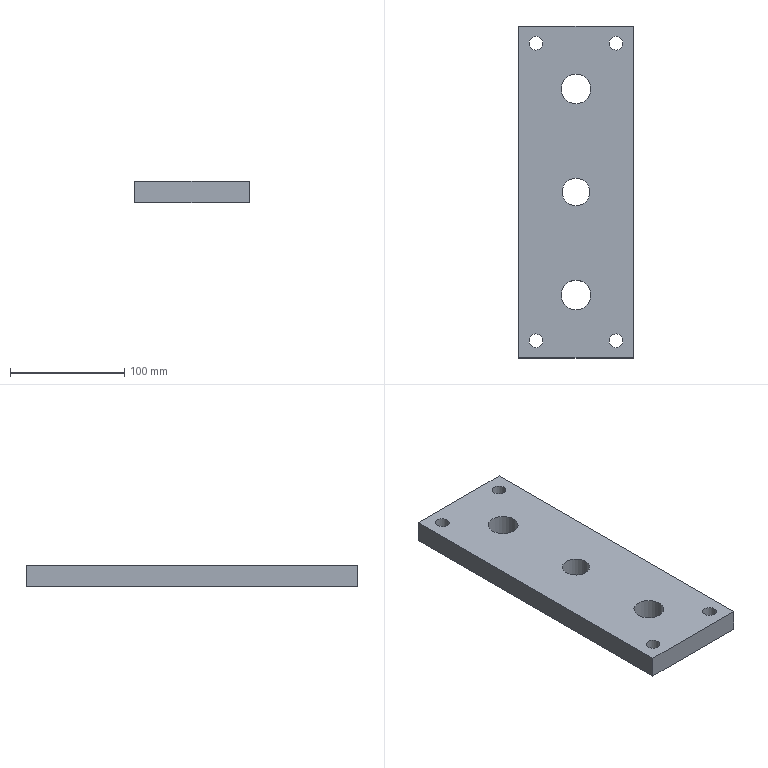Part | NX | features solid 2 | 1 solid | 13 faces | box 100 x 290 x 19 mm | volume 513634 mm3 | cylinder 7 | plane 6 | commonest cylinder face diameters 12 x4 26 x2 24 x1
STEP:
#1=CARTESIAN_POINT('',(235.,-226.,-122.));
#2=VERTEX_POINT('',#1);
#3=CARTESIAN_POINT('',(235.,-220.,-122.));
#4=DIRECTION('',(0.,0.,1.));
#5=DIRECTION('',(0.,-1.,0.));
#6=AXIS2_PLACEMENT_3D('',#3,#4,#5);
#7=CIRCLE('',#6,6.);
#8=EDGE_CURVE('',#2,#2,#7,.T.);
#9=ORIENTED_EDGE('',*,*,#8,.F.);
#10=EDGE_LOOP('',(#9));
#11=FACE_BOUND('',#10,.T.);
#12=CARTESIAN_POINT('',(235.,46.,-122.));
#13=VERTEX_POINT('',#12);
#14=CARTESIAN_POINT('',(235.,40.,-122.));
#15=DIRECTION('',(0.,0.,-1.));
#16=DIRECTION('',(0.,1.,0.));
#17=AXIS2_PLACEMENT_3D('',#14,#15,#16);
#18=CIRCLE('',#17,6.);
#19=EDGE_CURVE('',#13,#13,#18,.T.);
#20=ORIENTED_EDGE('',*,*,#19,.T.);
#21=EDGE_LOOP('',(#20));
#22=FACE_BOUND('',#21,.T.);
#23=CARTESIAN_POINT('',(250.,-235.,-122.));
#24=VERTEX_POINT('',#23);
#25=CARTESIAN_POINT('',(150.,-235.,-122.));
#26=VERTEX_POINT('',#25);
#27=CARTESIAN_POINT('',(250.,-235.,-122.));
#28=DIRECTION('',(-1.,0.,0.));
#29=VECTOR('',#28,1000.);
#30=LINE('',#27,#29);
#31=EDGE_CURVE('',#24,#26,#30,.T.);
#32=ORIENTED_EDGE('',*,*,#31,.F.);
#33=CARTESIAN_POINT('',(250.,55.,-122.));
#34=VERTEX_POINT('',#33);
#35=CARTESIAN_POINT('',(250.,55.,-122.));
#36=DIRECTION('',(0.,-1.,0.));
#37=VECTOR('',#36,1000.);
#38=LINE('',#35,#37);
#39=EDGE_CURVE('',#34,#24,#38,.T.);
#40=ORIENTED_EDGE('',*,*,#39,.F.);
#41=CARTESIAN_POINT('',(150.,55.,-122.));
#42=VERTEX_POINT('',#41);
#43=CARTESIAN_POINT('',(150.,55.,-122.));
#44=DIRECTION('',(1.,0.,0.));
#45=VECTOR('',#44,1000.);
#46=LINE('',#43,#45);
#47=EDGE_CURVE('',#42,#34,#46,.T.);
#48=ORIENTED_EDGE('',*,*,#47,.F.);
#49=CARTESIAN_POINT('',(150.,-235.,-122.));
#50=DIRECTION('',(0.,1.,0.));
#51=VECTOR('',#50,1000.);
#52=LINE('',#49,#51);
#53=EDGE_CURVE('',#26,#42,#52,.T.);
#54=ORIENTED_EDGE('',*,*,#53,.F.);
#55=EDGE_LOOP('',(#32,#40,#48,#54));
#56=FACE_BOUND('',#55,.T.);
#57=CARTESIAN_POINT('',(200.,-193.,-122.));
#58=VERTEX_POINT('',#57);
#59=CARTESIAN_POINT('',(200.,-180.,-122.));
#60=DIRECTION('',(0.,0.,1.));
#61=DIRECTION('',(0.,-1.,0.));
#62=AXIS2_PLACEMENT_3D('',#59,#60,#61);
#63=CIRCLE('',#62,13.);
#64=EDGE_CURVE('',#58,#58,#63,.F.);
#65=ORIENTED_EDGE('',*,*,#64,.T.);
#66=EDGE_LOOP('',(#65));
#67=FACE_BOUND('',#66,.T.);
#68=CARTESIAN_POINT('',(200.,-102.,-122.));
#69=VERTEX_POINT('',#68);
#70=CARTESIAN_POINT('',(200.,-90.,-122.));
#71=DIRECTION('',(0.,0.,1.));
#72=DIRECTION('',(0.,-1.,0.));
#73=AXIS2_PLACEMENT_3D('',#70,#71,#72);
#74=CIRCLE('',#73,12.);
#75=EDGE_CURVE('',#69,#69,#74,.F.);
#76=ORIENTED_EDGE('',*,*,#75,.T.);
#77=EDGE_LOOP('',(#76));
#78=FACE_BOUND('',#77,.T.);
#79=CARTESIAN_POINT('',(165.,46.,-122.));
#80=VERTEX_POINT('',#79);
#81=CARTESIAN_POINT('',(165.,40.,-122.));
#82=DIRECTION('',(0.,0.,1.));
#83=DIRECTION('',(0.,1.,0.));
#84=AXIS2_PLACEMENT_3D('',#81,#82,#83);
#85=CIRCLE('',#84,6.);
#86=EDGE_CURVE('',#80,#80,#85,.T.);
#87=ORIENTED_EDGE('',*,*,#86,.F.);
#88=EDGE_LOOP('',(#87));
#89=FACE_BOUND('',#88,.T.);
#90=CARTESIAN_POINT('',(165.,-226.,-122.));
#91=VERTEX_POINT('',#90);
#92=CARTESIAN_POINT('',(165.,-220.,-122.));
#93=DIRECTION('',(0.,0.,-1.));
#94=DIRECTION('',(0.,-1.,0.));
#95=AXIS2_PLACEMENT_3D('',#92,#93,#94);
#96=CIRCLE('',#95,6.);
#97=EDGE_CURVE('',#91,#91,#96,.T.);
#98=ORIENTED_EDGE('',*,*,#97,.T.);
#99=EDGE_LOOP('',(#98));
#100=FACE_BOUND('',#99,.T.);
#101=CARTESIAN_POINT('',(200.,13.,-122.));
#102=VERTEX_POINT('',#101);
#103=CARTESIAN_POINT('',(200.,0.,-122.));
#104=DIRECTION('',(0.,0.,1.));
#105=DIRECTION('',(0.,1.,0.));
#106=AXIS2_PLACEMENT_3D('',#103,#104,#105);
#107=CIRCLE('',#106,13.);
#108=EDGE_CURVE('',#102,#102,#107,.T.);
#109=ORIENTED_EDGE('',*,*,#108,.F.);
#110=EDGE_LOOP('',(#109));
#111=FACE_BOUND('',#110,.T.);
#112=CARTESIAN_POINT('',(250.,-235.,-122.));
#113=DIRECTION('',(0.,0.,1.));
#114=DIRECTION('',(0.,-1.,0.));
#115=AXIS2_PLACEMENT_3D('',#112,#113,#114);
#116=PLANE('',#115);
#117=ADVANCED_FACE('',(#11,#22,#56,#67,#78,#89,#100,#111),#116,.T.);
#118=CARTESIAN_POINT('',(235.,-226.,-141.));
#119=VERTEX_POINT('',#118);
#120=CARTESIAN_POINT('',(235.,-220.,-141.));
#121=DIRECTION('',(0.,0.,1.));
#122=DIRECTION('',(0.,-1.,0.));
#123=AXIS2_PLACEMENT_3D('',#120,#121,#122);
#124=CIRCLE('',#123,6.);
#125=EDGE_CURVE('',#119,#119,#124,.T.);
#126=ORIENTED_EDGE('',*,*,#125,.T.);
#127=EDGE_LOOP('',(#126));
#128=FACE_BOUND('',#127,.T.);
#129=CARTESIAN_POINT('',(235.,46.,-141.));
#130=VERTEX_POINT('',#129);
#131=CARTESIAN_POINT('',(235.,40.,-141.));
#132=DIRECTION('',(0.,0.,-1.));
#133=DIRECTION('',(0.,1.,0.));
#134=AXIS2_PLACEMENT_3D('',#131,#132,#133);
#135=CIRCLE('',#134,6.);
#136=EDGE_CURVE('',#130,#130,#135,.T.);
#137=ORIENTED_EDGE('',*,*,#136,.F.);
#138=EDGE_LOOP('',(#137));
#139=FACE_BOUND('',#138,.T.);
#140=CARTESIAN_POINT('',(250.,-235.,-141.));
#141=VERTEX_POINT('',#140);
#142=CARTESIAN_POINT('',(150.,-235.,-141.));
#143=VERTEX_POINT('',#142);
#144=CARTESIAN_POINT('',(250.,-235.,-141.));
#145=DIRECTION('',(-1.,0.,0.));
#146=VECTOR('',#145,1000.);
#147=LINE('',#144,#146);
#148=EDGE_CURVE('',#141,#143,#147,.T.);
#149=ORIENTED_EDGE('',*,*,#148,.T.);
#150=CARTESIAN_POINT('',(150.,55.,-141.));
#151=VERTEX_POINT('',#150);
#152=CARTESIAN_POINT('',(150.,-235.,-141.));
#153=DIRECTION('',(0.,1.,0.));
#154=VECTOR('',#153,1000.);
#155=LINE('',#152,#154);
#156=EDGE_CURVE('',#143,#151,#155,.T.);
#157=ORIENTED_EDGE('',*,*,#156,.T.);
#158=CARTESIAN_POINT('',(250.,55.,-141.));
#159=VERTEX_POINT('',#158);
#160=CARTESIAN_POINT('',(150.,55.,-141.));
#161=DIRECTION('',(1.,0.,0.));
#162=VECTOR('',#161,1000.);
#163=LINE('',#160,#162);
#164=EDGE_CURVE('',#151,#159,#163,.T.);
#165=ORIENTED_EDGE('',*,*,#164,.T.);
#166=CARTESIAN_POINT('',(250.,55.,-141.));
#167=DIRECTION('',(0.,-1.,0.));
#168=VECTOR('',#167,1000.);
#169=LINE('',#166,#168);
#170=EDGE_CURVE('',#159,#141,#169,.T.);
#171=ORIENTED_EDGE('',*,*,#170,.T.);
#172=EDGE_LOOP('',(#149,#157,#165,#171));
#173=FACE_BOUND('',#172,.T.);
#174=CARTESIAN_POINT('',(200.,-193.,-141.));
#175=VERTEX_POINT('',#174);
#176=CARTESIAN_POINT('',(200.,-180.,-141.));
#177=DIRECTION('',(0.,0.,1.));
#178=DIRECTION('',(0.,-1.,0.));
#179=AXIS2_PLACEMENT_3D('',#176,#177,#178);
#180=CIRCLE('',#179,13.);
#181=EDGE_CURVE('',#175,#175,#180,.F.);
#182=ORIENTED_EDGE('',*,*,#181,.F.);
#183=EDGE_LOOP('',(#182));
#184=FACE_BOUND('',#183,.T.);
#185=CARTESIAN_POINT('',(200.,-102.,-141.));
#186=VERTEX_POINT('',#185);
#187=CARTESIAN_POINT('',(200.,-90.,-141.));
#188=DIRECTION('',(0.,0.,1.));
#189=DIRECTION('',(0.,-1.,0.));
#190=AXIS2_PLACEMENT_3D('',#187,#188,#189);
#191=CIRCLE('',#190,12.);
#192=EDGE_CURVE('',#186,#186,#191,.F.);
#193=ORIENTED_EDGE('',*,*,#192,.F.);
#194=EDGE_LOOP('',(#193));
#195=FACE_BOUND('',#194,.T.);
#196=CARTESIAN_POINT('',(165.,46.,-141.));
#197=VERTEX_POINT('',#196);
#198=CARTESIAN_POINT('',(165.,40.,-141.));
#199=DIRECTION('',(0.,0.,1.));
#200=DIRECTION('',(0.,1.,0.));
#201=AXIS2_PLACEMENT_3D('',#198,#199,#200);
#202=CIRCLE('',#201,6.);
#203=EDGE_CURVE('',#197,#197,#202,.T.);
#204=ORIENTED_EDGE('',*,*,#203,.T.);
#205=EDGE_LOOP('',(#204));
#206=FACE_BOUND('',#205,.T.);
#207=CARTESIAN_POINT('',(165.,-226.,-141.));
#208=VERTEX_POINT('',#207);
#209=CARTESIAN_POINT('',(165.,-220.,-141.));
#210=DIRECTION('',(0.,0.,-1.));
#211=DIRECTION('',(0.,-1.,0.));
#212=AXIS2_PLACEMENT_3D('',#209,#210,#211);
#213=CIRCLE('',#212,6.);
#214=EDGE_CURVE('',#208,#208,#213,.T.);
#215=ORIENTED_EDGE('',*,*,#214,.F.);
#216=EDGE_LOOP('',(#215));
#217=FACE_BOUND('',#216,.T.);
#218=CARTESIAN_POINT('',(200.,13.,-141.));
#219=VERTEX_POINT('',#218);
#220=CARTESIAN_POINT('',(200.,0.,-141.));
#221=DIRECTION('',(0.,0.,1.));
#222=DIRECTION('',(0.,1.,0.));
#223=AXIS2_PLACEMENT_3D('',#220,#221,#222);
#224=CIRCLE('',#223,13.);
#225=EDGE_CURVE('',#219,#219,#224,.T.);
#226=ORIENTED_EDGE('',*,*,#225,.T.);
#227=EDGE_LOOP('',(#226));
#228=FACE_BOUND('',#227,.T.);
#229=CARTESIAN_POINT('',(250.,-235.,-141.));
#230=DIRECTION('',(0.,0.,1.));
#231=DIRECTION('',(0.,-1.,0.));
#232=AXIS2_PLACEMENT_3D('',#229,#230,#231);
#233=PLANE('',#232);
#234=ADVANCED_FACE('',(#128,#139,#173,#184,#195,#206,#217,#228),#233,.F.);
#235=ORIENTED_EDGE('',*,*,#148,.F.);
#236=CARTESIAN_POINT('',(250.,-235.,-122.));
#237=DIRECTION('',(0.,0.,-1.));
#238=VECTOR('',#237,1000.);
#239=LINE('',#236,#238);
#240=EDGE_CURVE('',#24,#141,#239,.T.);
#241=ORIENTED_EDGE('',*,*,#240,.F.);
#242=ORIENTED_EDGE('',*,*,#31,.T.);
#243=CARTESIAN_POINT('',(150.,-235.,-122.));
#244=DIRECTION('',(0.,0.,-1.));
#245=VECTOR('',#244,1000.);
#246=LINE('',#243,#245);
#247=EDGE_CURVE('',#26,#143,#246,.T.);
#248=ORIENTED_EDGE('',*,*,#247,.T.);
#249=EDGE_LOOP('',(#235,#241,#242,#248));
#250=FACE_BOUND('',#249,.T.);
#251=CARTESIAN_POINT('',(250.,-235.,-122.));
#252=DIRECTION('',(0.,-1.,0.));
#253=DIRECTION('',(0.,0.,-1.));
#254=AXIS2_PLACEMENT_3D('',#251,#252,#253);
#255=PLANE('',#254);
#256=ADVANCED_FACE('',(#250),#255,.T.);
#257=ORIENTED_EDGE('',*,*,#156,.F.);
#258=ORIENTED_EDGE('',*,*,#247,.F.);
#259=ORIENTED_EDGE('',*,*,#53,.T.);
#260=CARTESIAN_POINT('',(150.,55.,-122.));
#261=DIRECTION('',(0.,0.,-1.));
#262=VECTOR('',#261,1000.);
#263=LINE('',#260,#262);
#264=EDGE_CURVE('',#42,#151,#263,.T.);
#265=ORIENTED_EDGE('',*,*,#264,.T.);
#266=EDGE_LOOP('',(#257,#258,#259,#265));
#267=FACE_BOUND('',#266,.T.);
#268=CARTESIAN_POINT('',(150.,-235.,-122.));
#269=DIRECTION('',(-1.,0.,0.));
#270=DIRECTION('',(0.,-1.,0.));
#271=AXIS2_PLACEMENT_3D('',#268,#269,#270);
#272=PLANE('',#271);
#273=ADVANCED_FACE('',(#267),#272,.T.);
#274=ORIENTED_EDGE('',*,*,#164,.F.);
#275=ORIENTED_EDGE('',*,*,#264,.F.);
#276=ORIENTED_EDGE('',*,*,#47,.T.);
#277=CARTESIAN_POINT('',(250.,55.,-122.));
#278=DIRECTION('',(0.,0.,-1.));
#279=VECTOR('',#278,1000.);
#280=LINE('',#277,#279);
#281=EDGE_CURVE('',#34,#159,#280,.T.);
#282=ORIENTED_EDGE('',*,*,#281,.T.);
#283=EDGE_LOOP('',(#274,#275,#276,#282));
#284=FACE_BOUND('',#283,.T.);
#285=CARTESIAN_POINT('',(150.,55.,-122.));
#286=DIRECTION('',(0.,1.,0.));
#287=DIRECTION('',(0.,0.,1.));
#288=AXIS2_PLACEMENT_3D('',#285,#286,#287);
#289=PLANE('',#288);
#290=ADVANCED_FACE('',(#284),#289,.T.);
#291=ORIENTED_EDGE('',*,*,#19,.F.);
#292=EDGE_LOOP('',(#291));
#293=FACE_BOUND('',#292,.T.);
#294=ORIENTED_EDGE('',*,*,#136,.T.);
#295=EDGE_LOOP('',(#294));
#296=FACE_BOUND('',#295,.T.);
#297=CARTESIAN_POINT('',(235.,40.,-122.));
#298=DIRECTION('',(0.,0.,-1.));
#299=DIRECTION('',(0.,1.,0.));
#300=AXIS2_PLACEMENT_3D('',#297,#298,#299);
#301=CYLINDRICAL_SURFACE('',#300,6.);
#302=ADVANCED_FACE('',(#293,#296),#301,.F.);
#303=ORIENTED_EDGE('',*,*,#170,.F.);
#304=ORIENTED_EDGE('',*,*,#281,.F.);
#305=ORIENTED_EDGE('',*,*,#39,.T.);
#306=ORIENTED_EDGE('',*,*,#240,.T.);
#307=EDGE_LOOP('',(#303,#304,#305,#306));
#308=FACE_BOUND('',#307,.T.);
#309=CARTESIAN_POINT('',(250.,55.,-122.));
#310=DIRECTION('',(1.,0.,0.));
#311=DIRECTION('',(0.,0.,1.));
#312=AXIS2_PLACEMENT_3D('',#309,#310,#311);
#313=PLANE('',#312);
#314=ADVANCED_FACE('',(#308),#313,.T.);
#315=ORIENTED_EDGE('',*,*,#64,.F.);
#316=EDGE_LOOP('',(#315));
#317=FACE_BOUND('',#316,.T.);
#318=ORIENTED_EDGE('',*,*,#181,.T.);
#319=EDGE_LOOP('',(#318));
#320=FACE_BOUND('',#319,.T.);
#321=CARTESIAN_POINT('',(200.,-180.,-122.));
#322=DIRECTION('',(0.,0.,-1.));
#323=DIRECTION('',(0.,1.,0.));
#324=AXIS2_PLACEMENT_3D('',#321,#322,#323);
#325=CYLINDRICAL_SURFACE('',#324,13.);
#326=ADVANCED_FACE('',(#317,#320),#325,.F.);
#327=ORIENTED_EDGE('',*,*,#75,.F.);
#328=EDGE_LOOP('',(#327));
#329=FACE_BOUND('',#328,.T.);
#330=ORIENTED_EDGE('',*,*,#192,.T.);
#331=EDGE_LOOP('',(#330));
#332=FACE_BOUND('',#331,.T.);
#333=CARTESIAN_POINT('',(200.,-90.,-122.));
#334=DIRECTION('',(0.,0.,-1.));
#335=DIRECTION('',(0.,1.,0.));
#336=AXIS2_PLACEMENT_3D('',#333,#334,#335);
#337=CYLINDRICAL_SURFACE('',#336,12.);
#338=ADVANCED_FACE('',(#329,#332),#337,.F.);
#339=ORIENTED_EDGE('',*,*,#86,.T.);
#340=EDGE_LOOP('',(#339));
#341=FACE_BOUND('',#340,.T.);
#342=ORIENTED_EDGE('',*,*,#203,.F.);
#343=EDGE_LOOP('',(#342));
#344=FACE_BOUND('',#343,.T.);
#345=CARTESIAN_POINT('',(165.,40.,-122.));
#346=DIRECTION('',(0.,0.,-1.));
#347=DIRECTION('',(0.,1.,0.));
#348=AXIS2_PLACEMENT_3D('',#345,#346,#347);
#349=CYLINDRICAL_SURFACE('',#348,6.);
#350=ADVANCED_FACE('',(#341,#344),#349,.F.);
#351=ORIENTED_EDGE('',*,*,#97,.F.);
#352=EDGE_LOOP('',(#351));
#353=FACE_BOUND('',#352,.T.);
#354=ORIENTED_EDGE('',*,*,#214,.T.);
#355=EDGE_LOOP('',(#354));
#356=FACE_BOUND('',#355,.T.);
#357=CARTESIAN_POINT('',(165.,-220.,-122.));
#358=DIRECTION('',(0.,0.,-1.));
#359=DIRECTION('',(0.,1.,0.));
#360=AXIS2_PLACEMENT_3D('',#357,#358,#359);
#361=CYLINDRICAL_SURFACE('',#360,6.);
#362=ADVANCED_FACE('',(#353,#356),#361,.F.);
#363=ORIENTED_EDGE('',*,*,#8,.T.);
#364=EDGE_LOOP('',(#363));
#365=FACE_BOUND('',#364,.T.);
#366=ORIENTED_EDGE('',*,*,#125,.F.);
#367=EDGE_LOOP('',(#366));
#368=FACE_BOUND('',#367,.T.);
#369=CARTESIAN_POINT('',(235.,-220.,-122.));
#370=DIRECTION('',(0.,0.,-1.));
#371=DIRECTION('',(0.,1.,0.));
#372=AXIS2_PLACEMENT_3D('',#369,#370,#371);
#373=CYLINDRICAL_SURFACE('',#372,6.);
#374=ADVANCED_FACE('',(#365,#368),#373,.F.);
#375=ORIENTED_EDGE('',*,*,#225,.F.);
#376=EDGE_LOOP('',(#375));
#377=FACE_BOUND('',#376,.T.);
#378=ORIENTED_EDGE('',*,*,#108,.T.);
#379=EDGE_LOOP('',(#378));
#380=FACE_BOUND('',#379,.T.);
#381=CARTESIAN_POINT('',(200.,0.,-141.));
#382=DIRECTION('',(0.,0.,1.));
#383=DIRECTION('',(0.,1.,0.));
#384=AXIS2_PLACEMENT_3D('',#381,#382,#383);
#385=CYLINDRICAL_SURFACE('',#384,13.);
#386=ADVANCED_FACE('',(#377,#380),#385,.F.);
#387=CLOSED_SHELL('',(#117,#234,#256,#273,#290,#302,#314,#326,#338,#350,#362,#374,#386));
#388=MANIFOLD_SOLID_BREP('',#387);
#389=(LENGTH_UNIT()NAMED_UNIT(*)SI_UNIT(.MILLI.,.METRE.));
#390=UNCERTAINTY_MEASURE_WITH_UNIT(LENGTH_MEASURE(0.00001),#389,'','');
#391=(NAMED_UNIT(*)PLANE_ANGLE_UNIT()SI_UNIT($,.RADIAN.));
#392=(NAMED_UNIT(*)SI_UNIT($,.STERADIAN.)SOLID_ANGLE_UNIT());
#393=(GEOMETRIC_REPRESENTATION_CONTEXT(3)GLOBAL_UNCERTAINTY_ASSIGNED_CONTEXT((#390))GLOBAL_UNIT_ASSIGNED_CONTEXT((#389,#391,#392))REPRESENTATION_CONTEXT('',''));
#394=ADVANCED_BREP_SHAPE_REPRESENTATION('',(#388),#393);